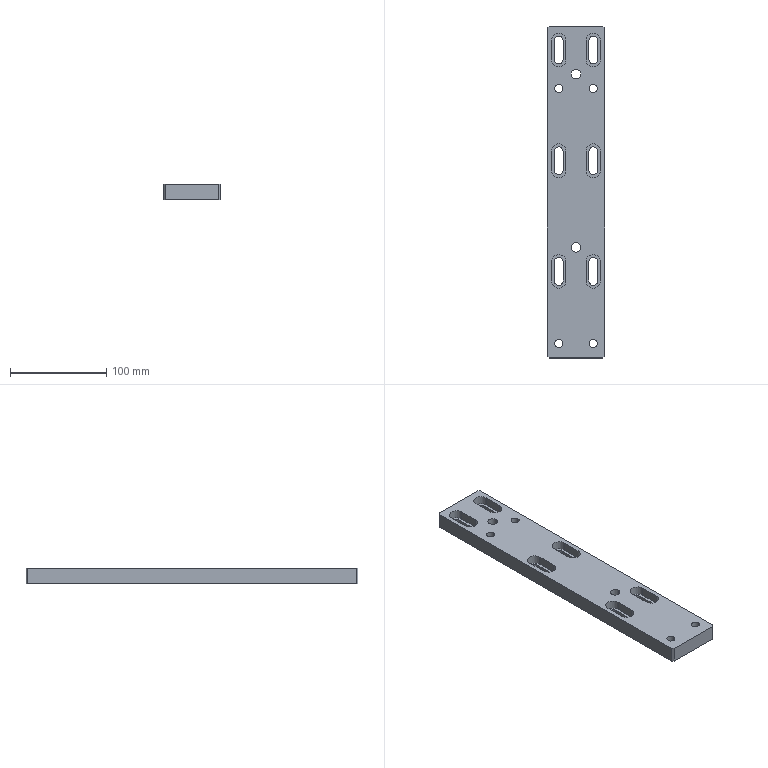Part | SolidWorks | features RefAxis 4, HoleWzd 3, ICE 2, Chamfer 1, Extrusion 1 | 1 solid | 76 faces | box 60 x 345 x 16 mm | volume 288953 mm3 | plane 40 | cylinder 36 | commonest cylinder face diameters 9 x12 15 x12 8.5 x8 10 x4